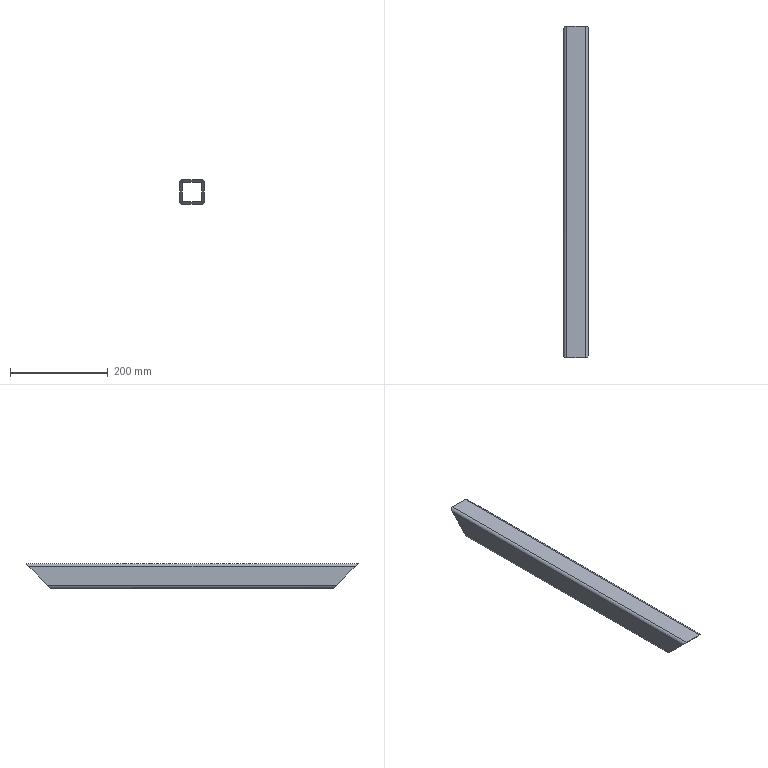Part | SolidWorks | features Extrusion 1, ICE 1 | 1 solid | 18 faces | box 50 x 680 x 50 mm | volume 548072 mm3 | plane 10 | cylinder 8 | commonest cylinder face diameters 2 x4 12 x4
STEP:
#1=CARTESIAN_POINT('',(-20.,674.,6.278));
#2=VERTEX_POINT('',#1);
#3=CARTESIAN_POINT('',(-20.,636.,-31.722));
#4=VERTEX_POINT('',#3);
#5=CARTESIAN_POINT('',(-20.,677.,9.278));
#6=DIRECTION('',(0.,-0.7071,-0.7071));
#7=VECTOR('',#6,1000.);
#8=LINE('',#5,#7);
#9=EDGE_CURVE('',#2,#4,#8,.T.);
#10=ORIENTED_EDGE('',*,*,#9,.F.);
#11=CARTESIAN_POINT('',(-20.,6.,6.278));
#12=VERTEX_POINT('',#11);
#13=CARTESIAN_POINT('',(-20.,680.,6.278));
#14=DIRECTION('',(0.,-1.,0.));
#15=VECTOR('',#14,1000.);
#16=LINE('',#13,#15);
#17=EDGE_CURVE('',#2,#12,#16,.T.);
#18=ORIENTED_EDGE('',*,*,#17,.T.);
#19=CARTESIAN_POINT('',(-20.,44.,-31.722));
#20=VERTEX_POINT('',#19);
#21=CARTESIAN_POINT('',(-20.,343.,-330.722));
#22=DIRECTION('',(0.,-0.7071,0.7071));
#23=VECTOR('',#22,1000.);
#24=LINE('',#21,#23);
#25=EDGE_CURVE('',#20,#12,#24,.T.);
#26=ORIENTED_EDGE('',*,*,#25,.F.);
#27=CARTESIAN_POINT('',(-20.,680.,-31.722));
#28=DIRECTION('',(0.,-1.,0.));
#29=VECTOR('',#28,1000.);
#30=LINE('',#27,#29);
#31=EDGE_CURVE('',#4,#20,#30,.T.);
#32=ORIENTED_EDGE('',*,*,#31,.F.);
#33=EDGE_LOOP('',(#10,#18,#26,#32));
#34=FACE_OUTER_BOUND('',#33,.T.);
#35=CARTESIAN_POINT('',(-20.,680.,6.278));
#36=DIRECTION('',(1.,0.,0.));
#37=DIRECTION('',(0.,0.,-1.));
#38=AXIS2_PLACEMENT_3D('',#35,#36,#37);
#39=PLANE('',#38);
#40=ADVANCED_FACE('',(#34),#39,.T.);
#41=CARTESIAN_POINT('',(-19.,635.,-32.722));
#42=VERTEX_POINT('',#41);
#43=CARTESIAN_POINT('',(-20.,636.,-31.722));
#44=CARTESIAN_POINT('',(-20.,635.414,-32.308));
#45=CARTESIAN_POINT('',(-19.586,635.,-32.722));
#46=CARTESIAN_POINT('',(-19.,635.,-32.722));
#47=(BOUNDED_CURVE()B_SPLINE_CURVE(3,(#43,#44,#45,#46),.UNSPECIFIED.,.F.,.F.)B_SPLINE_CURVE_WITH_KNOTS((4,4),(4.712,6.283),.UNSPECIFIED.)CURVE()GEOMETRIC_REPRESENTATION_ITEM()RATIONAL_B_SPLINE_CURVE((1.,0.8047,0.8047,1.))REPRESENTATION_ITEM(''));
#48=EDGE_CURVE('',#4,#42,#47,.T.);
#49=ORIENTED_EDGE('',*,*,#48,.F.);
#50=ORIENTED_EDGE('',*,*,#31,.T.);
#51=CARTESIAN_POINT('',(-19.,45.,-32.722));
#52=VERTEX_POINT('',#51);
#53=CARTESIAN_POINT('',(-19.,45.,-32.722));
#54=CARTESIAN_POINT('',(-19.586,45.,-32.722));
#55=CARTESIAN_POINT('',(-20.,44.586,-32.308));
#56=CARTESIAN_POINT('',(-20.,44.,-31.722));
#57=(BOUNDED_CURVE()B_SPLINE_CURVE(3,(#53,#54,#55,#56),.UNSPECIFIED.,.F.,.F.)B_SPLINE_CURVE_WITH_KNOTS((4,4),(3.142,4.712),.UNSPECIFIED.)CURVE()GEOMETRIC_REPRESENTATION_ITEM()RATIONAL_B_SPLINE_CURVE((1.,0.8047,0.8047,1.))REPRESENTATION_ITEM(''));
#58=EDGE_CURVE('',#52,#20,#57,.T.);
#59=ORIENTED_EDGE('',*,*,#58,.F.);
#60=CARTESIAN_POINT('',(-19.,680.,-32.722));
#61=DIRECTION('',(0.,-1.,0.));
#62=VECTOR('',#61,1000.);
#63=LINE('',#60,#62);
#64=EDGE_CURVE('',#42,#52,#63,.T.);
#65=ORIENTED_EDGE('',*,*,#64,.F.);
#66=EDGE_LOOP('',(#49,#50,#59,#65));
#67=FACE_OUTER_BOUND('',#66,.T.);
#68=CARTESIAN_POINT('',(-19.,680.,-31.722));
#69=DIRECTION('',(0.,-1.,0.));
#70=DIRECTION('',(0.,0.,-1.));
#71=AXIS2_PLACEMENT_3D('',#68,#69,#70);
#72=CYLINDRICAL_SURFACE('',#71,1.);
#73=ADVANCED_FACE('',(#67),#72,.F.);
#74=CARTESIAN_POINT('',(19.,635.,-32.722));
#75=VERTEX_POINT('',#74);
#76=CARTESIAN_POINT('',(-19.,635.,-32.722));
#77=DIRECTION('',(1.,0.,0.));
#78=VECTOR('',#77,1000.);
#79=LINE('',#76,#78);
#80=EDGE_CURVE('',#42,#75,#79,.T.);
#81=ORIENTED_EDGE('',*,*,#80,.F.);
#82=ORIENTED_EDGE('',*,*,#64,.T.);
#83=CARTESIAN_POINT('',(19.,45.,-32.722));
#84=VERTEX_POINT('',#83);
#85=CARTESIAN_POINT('',(-19.,45.,-32.722));
#86=DIRECTION('',(-1.,0.,0.));
#87=VECTOR('',#86,1000.);
#88=LINE('',#85,#87);
#89=EDGE_CURVE('',#84,#52,#88,.T.);
#90=ORIENTED_EDGE('',*,*,#89,.F.);
#91=CARTESIAN_POINT('',(19.,680.,-32.722));
#92=DIRECTION('',(0.,-1.,0.));
#93=VECTOR('',#92,1000.);
#94=LINE('',#91,#93);
#95=EDGE_CURVE('',#75,#84,#94,.T.);
#96=ORIENTED_EDGE('',*,*,#95,.F.);
#97=EDGE_LOOP('',(#81,#82,#90,#96));
#98=FACE_OUTER_BOUND('',#97,.T.);
#99=CARTESIAN_POINT('',(-19.,680.,-32.722));
#100=DIRECTION('',(0.,0.,1.));
#101=DIRECTION('',(1.,0.,0.));
#102=AXIS2_PLACEMENT_3D('',#99,#100,#101);
#103=PLANE('',#102);
#104=ADVANCED_FACE('',(#98),#103,.T.);
#105=CARTESIAN_POINT('',(20.,636.,-31.722));
#106=VERTEX_POINT('',#105);
#107=CARTESIAN_POINT('',(19.,635.,-32.722));
#108=CARTESIAN_POINT('',(19.586,635.,-32.722));
#109=CARTESIAN_POINT('',(20.,635.414,-32.308));
#110=CARTESIAN_POINT('',(20.,636.,-31.722));
#111=(BOUNDED_CURVE()B_SPLINE_CURVE(3,(#107,#108,#109,#110),.UNSPECIFIED.,.F.,.F.)B_SPLINE_CURVE_WITH_KNOTS((4,4),(0.,1.571),.UNSPECIFIED.)CURVE()GEOMETRIC_REPRESENTATION_ITEM()RATIONAL_B_SPLINE_CURVE((1.,0.8047,0.8047,1.))REPRESENTATION_ITEM(''));
#112=EDGE_CURVE('',#75,#106,#111,.T.);
#113=ORIENTED_EDGE('',*,*,#112,.F.);
#114=ORIENTED_EDGE('',*,*,#95,.T.);
#115=CARTESIAN_POINT('',(20.,44.,-31.722));
#116=VERTEX_POINT('',#115);
#117=CARTESIAN_POINT('',(20.,44.,-31.722));
#118=CARTESIAN_POINT('',(20.,44.586,-32.308));
#119=CARTESIAN_POINT('',(19.586,45.,-32.722));
#120=CARTESIAN_POINT('',(19.,45.,-32.722));
#121=(BOUNDED_CURVE()B_SPLINE_CURVE(3,(#117,#118,#119,#120),.UNSPECIFIED.,.F.,.F.)B_SPLINE_CURVE_WITH_KNOTS((4,4),(1.571,3.142),.UNSPECIFIED.)CURVE()GEOMETRIC_REPRESENTATION_ITEM()RATIONAL_B_SPLINE_CURVE((1.,0.8047,0.8047,1.))REPRESENTATION_ITEM(''));
#122=EDGE_CURVE('',#116,#84,#121,.T.);
#123=ORIENTED_EDGE('',*,*,#122,.F.);
#124=CARTESIAN_POINT('',(20.,680.,-31.722));
#125=DIRECTION('',(0.,-1.,0.));
#126=VECTOR('',#125,1000.);
#127=LINE('',#124,#126);
#128=EDGE_CURVE('',#106,#116,#127,.T.);
#129=ORIENTED_EDGE('',*,*,#128,.F.);
#130=EDGE_LOOP('',(#113,#114,#123,#129));
#131=FACE_OUTER_BOUND('',#130,.T.);
#132=CARTESIAN_POINT('',(19.,680.,-31.722));
#133=DIRECTION('',(0.,-1.,0.));
#134=DIRECTION('',(0.,0.,-1.));
#135=AXIS2_PLACEMENT_3D('',#132,#133,#134);
#136=CYLINDRICAL_SURFACE('',#135,1.);
#137=ADVANCED_FACE('',(#131),#136,.F.);
#138=CARTESIAN_POINT('',(20.,674.,6.278));
#139=VERTEX_POINT('',#138);
#140=CARTESIAN_POINT('',(20.,677.,9.278));
#141=DIRECTION('',(0.,0.7071,0.7071));
#142=VECTOR('',#141,1000.);
#143=LINE('',#140,#142);
#144=EDGE_CURVE('',#106,#139,#143,.T.);
#145=ORIENTED_EDGE('',*,*,#144,.F.);
#146=ORIENTED_EDGE('',*,*,#128,.T.);
#147=CARTESIAN_POINT('',(20.,6.,6.278));
#148=VERTEX_POINT('',#147);
#149=CARTESIAN_POINT('',(20.,343.,-330.722));
#150=DIRECTION('',(0.,0.7071,-0.7071));
#151=VECTOR('',#150,1000.);
#152=LINE('',#149,#151);
#153=EDGE_CURVE('',#148,#116,#152,.T.);
#154=ORIENTED_EDGE('',*,*,#153,.F.);
#155=CARTESIAN_POINT('',(20.,680.,6.278));
#156=DIRECTION('',(0.,-1.,0.));
#157=VECTOR('',#156,1000.);
#158=LINE('',#155,#157);
#159=EDGE_CURVE('',#139,#148,#158,.T.);
#160=ORIENTED_EDGE('',*,*,#159,.F.);
#161=EDGE_LOOP('',(#145,#146,#154,#160));
#162=FACE_OUTER_BOUND('',#161,.T.);
#163=CARTESIAN_POINT('',(20.,680.,6.278));
#164=DIRECTION('',(-1.,0.,0.));
#165=DIRECTION('',(0.,0.,1.));
#166=AXIS2_PLACEMENT_3D('',#163,#164,#165);
#167=PLANE('',#166);
#168=ADVANCED_FACE('',(#162),#167,.T.);
#169=CARTESIAN_POINT('',(19.,675.,7.278));
#170=VERTEX_POINT('',#169);
#171=CARTESIAN_POINT('',(20.,674.,6.278));
#172=CARTESIAN_POINT('',(20.,674.586,6.864));
#173=CARTESIAN_POINT('',(19.586,675.,7.278));
#174=CARTESIAN_POINT('',(19.,675.,7.278));
#175=(BOUNDED_CURVE()B_SPLINE_CURVE(3,(#171,#172,#173,#174),.UNSPECIFIED.,.F.,.F.)B_SPLINE_CURVE_WITH_KNOTS((4,4),(1.571,3.142),.UNSPECIFIED.)CURVE()GEOMETRIC_REPRESENTATION_ITEM()RATIONAL_B_SPLINE_CURVE((1.,0.8047,0.8047,1.))REPRESENTATION_ITEM(''));
#176=EDGE_CURVE('',#139,#170,#175,.T.);
#177=ORIENTED_EDGE('',*,*,#176,.F.);
#178=ORIENTED_EDGE('',*,*,#159,.T.);
#179=CARTESIAN_POINT('',(19.,5.,7.278));
#180=VERTEX_POINT('',#179);
#181=CARTESIAN_POINT('',(19.,5.,7.278));
#182=CARTESIAN_POINT('',(19.586,5.,7.278));
#183=CARTESIAN_POINT('',(20.,5.414,6.864));
#184=CARTESIAN_POINT('',(20.,6.,6.278));
#185=(BOUNDED_CURVE()B_SPLINE_CURVE(3,(#181,#182,#183,#184),.UNSPECIFIED.,.F.,.F.)B_SPLINE_CURVE_WITH_KNOTS((4,4),(0.,1.571),.UNSPECIFIED.)CURVE()GEOMETRIC_REPRESENTATION_ITEM()RATIONAL_B_SPLINE_CURVE((1.,0.8047,0.8047,1.))REPRESENTATION_ITEM(''));
#186=EDGE_CURVE('',#180,#148,#185,.T.);
#187=ORIENTED_EDGE('',*,*,#186,.F.);
#188=CARTESIAN_POINT('',(19.,680.,7.278));
#189=DIRECTION('',(0.,-1.,0.));
#190=VECTOR('',#189,1000.);
#191=LINE('',#188,#190);
#192=EDGE_CURVE('',#170,#180,#191,.T.);
#193=ORIENTED_EDGE('',*,*,#192,.F.);
#194=EDGE_LOOP('',(#177,#178,#187,#193));
#195=FACE_OUTER_BOUND('',#194,.T.);
#196=CARTESIAN_POINT('',(19.,680.,6.278));
#197=DIRECTION('',(0.,-1.,0.));
#198=DIRECTION('',(0.,0.,-1.));
#199=AXIS2_PLACEMENT_3D('',#196,#197,#198);
#200=CYLINDRICAL_SURFACE('',#199,1.);
#201=ADVANCED_FACE('',(#195),#200,.F.);
#202=CARTESIAN_POINT('',(-19.,675.,7.278));
#203=VERTEX_POINT('',#202);
#204=CARTESIAN_POINT('',(-19.,675.,7.278));
#205=DIRECTION('',(-1.,0.,0.));
#206=VECTOR('',#205,1000.);
#207=LINE('',#204,#206);
#208=EDGE_CURVE('',#170,#203,#207,.T.);
#209=ORIENTED_EDGE('',*,*,#208,.F.);
#210=ORIENTED_EDGE('',*,*,#192,.T.);
#211=CARTESIAN_POINT('',(-19.,5.,7.278));
#212=VERTEX_POINT('',#211);
#213=CARTESIAN_POINT('',(-19.,5.,7.278));
#214=DIRECTION('',(1.,0.,0.));
#215=VECTOR('',#214,1000.);
#216=LINE('',#213,#215);
#217=EDGE_CURVE('',#212,#180,#216,.T.);
#218=ORIENTED_EDGE('',*,*,#217,.F.);
#219=CARTESIAN_POINT('',(-19.,680.,7.278));
#220=DIRECTION('',(0.,-1.,0.));
#221=VECTOR('',#220,1000.);
#222=LINE('',#219,#221);
#223=EDGE_CURVE('',#203,#212,#222,.T.);
#224=ORIENTED_EDGE('',*,*,#223,.F.);
#225=EDGE_LOOP('',(#209,#210,#218,#224));
#226=FACE_OUTER_BOUND('',#225,.T.);
#227=CARTESIAN_POINT('',(-19.,680.,7.278));
#228=DIRECTION('',(0.,0.,-1.));
#229=DIRECTION('',(-1.,0.,0.));
#230=AXIS2_PLACEMENT_3D('',#227,#228,#229);
#231=PLANE('',#230);
#232=ADVANCED_FACE('',(#226),#231,.T.);
#233=CARTESIAN_POINT('',(-19.,675.,7.278));
#234=CARTESIAN_POINT('',(-19.586,675.,7.278));
#235=CARTESIAN_POINT('',(-20.,674.586,6.864));
#236=CARTESIAN_POINT('',(-20.,674.,6.278));
#237=(BOUNDED_CURVE()B_SPLINE_CURVE(3,(#233,#234,#235,#236),.UNSPECIFIED.,.F.,.F.)B_SPLINE_CURVE_WITH_KNOTS((4,4),(3.142,4.712),.UNSPECIFIED.)CURVE()GEOMETRIC_REPRESENTATION_ITEM()RATIONAL_B_SPLINE_CURVE((1.,0.8047,0.8047,1.))REPRESENTATION_ITEM(''));
#238=EDGE_CURVE('',#203,#2,#237,.T.);
#239=ORIENTED_EDGE('',*,*,#238,.F.);
#240=ORIENTED_EDGE('',*,*,#223,.T.);
#241=CARTESIAN_POINT('',(-20.,6.,6.278));
#242=CARTESIAN_POINT('',(-20.,5.414,6.864));
#243=CARTESIAN_POINT('',(-19.586,5.,7.278));
#244=CARTESIAN_POINT('',(-19.,5.,7.278));
#245=(BOUNDED_CURVE()B_SPLINE_CURVE(3,(#241,#242,#243,#244),.UNSPECIFIED.,.F.,.F.)B_SPLINE_CURVE_WITH_KNOTS((4,4),(4.712,6.283),.UNSPECIFIED.)CURVE()GEOMETRIC_REPRESENTATION_ITEM()RATIONAL_B_SPLINE_CURVE((1.,0.8047,0.8047,1.))REPRESENTATION_ITEM(''));
#246=EDGE_CURVE('',#12,#212,#245,.T.);
#247=ORIENTED_EDGE('',*,*,#246,.F.);
#248=ORIENTED_EDGE('',*,*,#17,.F.);
#249=EDGE_LOOP('',(#239,#240,#247,#248));
#250=FACE_OUTER_BOUND('',#249,.T.);
#251=CARTESIAN_POINT('',(-19.,680.,6.278));
#252=DIRECTION('',(0.,-1.,0.));
#253=DIRECTION('',(0.,0.,-1.));
#254=AXIS2_PLACEMENT_3D('',#251,#252,#253);
#255=CYLINDRICAL_SURFACE('',#254,1.);
#256=ADVANCED_FACE('',(#250),#255,.F.);
#257=ORIENTED_EDGE('',*,*,#246,.T.);
#258=ORIENTED_EDGE('',*,*,#217,.T.);
#259=ORIENTED_EDGE('',*,*,#186,.T.);
#260=ORIENTED_EDGE('',*,*,#153,.T.);
#261=ORIENTED_EDGE('',*,*,#122,.T.);
#262=ORIENTED_EDGE('',*,*,#89,.T.);
#263=ORIENTED_EDGE('',*,*,#58,.T.);
#264=ORIENTED_EDGE('',*,*,#25,.T.);
#265=EDGE_LOOP('',(#257,#258,#259,#260,#261,#262,#263,#264));
#266=FACE_BOUND('',#265,.T.);
#267=CARTESIAN_POINT('',(-25.,44.,-31.722));
#268=VERTEX_POINT('',#267);
#269=CARTESIAN_POINT('',(-25.,6.,6.278));
#270=VERTEX_POINT('',#269);
#271=CARTESIAN_POINT('',(-25.,0.,12.278));
#272=DIRECTION('',(0.,-0.7071,0.7071));
#273=VECTOR('',#272,1000.);
#274=LINE('',#271,#273);
#275=EDGE_CURVE('',#268,#270,#274,.T.);
#276=ORIENTED_EDGE('',*,*,#275,.F.);
#277=CARTESIAN_POINT('',(-19.,50.,-37.722));
#278=VERTEX_POINT('',#277);
#279=CARTESIAN_POINT('',(-19.,50.,-37.722));
#280=CARTESIAN_POINT('',(-22.515,50.,-37.722));
#281=CARTESIAN_POINT('',(-25.,47.515,-35.237));
#282=CARTESIAN_POINT('',(-25.,44.,-31.722));
#283=(BOUNDED_CURVE()B_SPLINE_CURVE(3,(#279,#280,#281,#282),.UNSPECIFIED.,.F.,.F.)B_SPLINE_CURVE_WITH_KNOTS((4,4),(3.142,4.712),.UNSPECIFIED.)CURVE()GEOMETRIC_REPRESENTATION_ITEM()RATIONAL_B_SPLINE_CURVE((1.,0.8047,0.8047,1.))REPRESENTATION_ITEM(''));
#284=EDGE_CURVE('',#278,#268,#283,.T.);
#285=ORIENTED_EDGE('',*,*,#284,.F.);
#286=CARTESIAN_POINT('',(19.,50.,-37.722));
#287=VERTEX_POINT('',#286);
#288=CARTESIAN_POINT('',(-25.,50.,-37.722));
#289=DIRECTION('',(1.,0.,0.));
#290=VECTOR('',#289,1000.);
#291=LINE('',#288,#290);
#292=EDGE_CURVE('',#278,#287,#291,.T.);
#293=ORIENTED_EDGE('',*,*,#292,.T.);
#294=CARTESIAN_POINT('',(25.,44.,-31.722));
#295=VERTEX_POINT('',#294);
#296=CARTESIAN_POINT('',(25.,44.,-31.722));
#297=CARTESIAN_POINT('',(25.,47.515,-35.237));
#298=CARTESIAN_POINT('',(22.515,50.,-37.722));
#299=CARTESIAN_POINT('',(19.,50.,-37.722));
#300=(BOUNDED_CURVE()B_SPLINE_CURVE(3,(#296,#297,#298,#299),.UNSPECIFIED.,.F.,.F.)B_SPLINE_CURVE_WITH_KNOTS((4,4),(1.571,3.142),.UNSPECIFIED.)CURVE()GEOMETRIC_REPRESENTATION_ITEM()RATIONAL_B_SPLINE_CURVE((1.,0.8047,0.8047,1.))REPRESENTATION_ITEM(''));
#301=EDGE_CURVE('',#295,#287,#300,.T.);
#302=ORIENTED_EDGE('',*,*,#301,.F.);
#303=CARTESIAN_POINT('',(25.,6.,6.278));
#304=VERTEX_POINT('',#303);
#305=CARTESIAN_POINT('',(25.,0.,12.278));
#306=DIRECTION('',(0.,-0.7071,0.7071));
#307=VECTOR('',#306,1000.);
#308=LINE('',#305,#307);
#309=EDGE_CURVE('',#295,#304,#308,.T.);
#310=ORIENTED_EDGE('',*,*,#309,.T.);
#311=CARTESIAN_POINT('',(19.,0.,12.278));
#312=VERTEX_POINT('',#311);
#313=CARTESIAN_POINT('',(19.,0.,12.278));
#314=CARTESIAN_POINT('',(22.515,0.,12.278));
#315=CARTESIAN_POINT('',(25.,2.485,9.793));
#316=CARTESIAN_POINT('',(25.,6.,6.278));
#317=(BOUNDED_CURVE()B_SPLINE_CURVE(3,(#313,#314,#315,#316),.UNSPECIFIED.,.F.,.F.)B_SPLINE_CURVE_WITH_KNOTS((4,4),(0.,1.571),.UNSPECIFIED.)CURVE()GEOMETRIC_REPRESENTATION_ITEM()RATIONAL_B_SPLINE_CURVE((1.,0.8047,0.8047,1.))REPRESENTATION_ITEM(''));
#318=EDGE_CURVE('',#312,#304,#317,.T.);
#319=ORIENTED_EDGE('',*,*,#318,.F.);
#320=CARTESIAN_POINT('',(-19.,0.,12.278));
#321=VERTEX_POINT('',#320);
#322=CARTESIAN_POINT('',(-19.,0.,12.278));
#323=DIRECTION('',(1.,0.,0.));
#324=VECTOR('',#323,1000.);
#325=LINE('',#322,#324);
#326=EDGE_CURVE('',#321,#312,#325,.T.);
#327=ORIENTED_EDGE('',*,*,#326,.F.);
#328=CARTESIAN_POINT('',(-25.,6.,6.278));
#329=CARTESIAN_POINT('',(-25.,2.485,9.793));
#330=CARTESIAN_POINT('',(-22.515,0.,12.278));
#331=CARTESIAN_POINT('',(-19.,0.,12.278));
#332=(BOUNDED_CURVE()B_SPLINE_CURVE(3,(#328,#329,#330,#331),.UNSPECIFIED.,.F.,.F.)B_SPLINE_CURVE_WITH_KNOTS((4,4),(4.712,6.283),.UNSPECIFIED.)CURVE()GEOMETRIC_REPRESENTATION_ITEM()RATIONAL_B_SPLINE_CURVE((1.,0.8047,0.8047,1.))REPRESENTATION_ITEM(''));
#333=EDGE_CURVE('',#270,#321,#332,.T.);
#334=ORIENTED_EDGE('',*,*,#333,.F.);
#335=EDGE_LOOP('',(#276,#285,#293,#302,#310,#319,#327,#334));
#336=FACE_OUTER_BOUND('',#335,.T.);
#337=CARTESIAN_POINT('',(-25.,0.,12.278));
#338=DIRECTION('',(0.,0.7071,0.7071));
#339=DIRECTION('',(0.,-0.7071,0.7071));
#340=AXIS2_PLACEMENT_3D('',#337,#338,#339);
#341=PLANE('',#340);
#342=ADVANCED_FACE('',(#266,#336),#341,.F.);
#343=ORIENTED_EDGE('',*,*,#238,.T.);
#344=ORIENTED_EDGE('',*,*,#9,.T.);
#345=ORIENTED_EDGE('',*,*,#48,.T.);
#346=ORIENTED_EDGE('',*,*,#80,.T.);
#347=ORIENTED_EDGE('',*,*,#112,.T.);
#348=ORIENTED_EDGE('',*,*,#144,.T.);
#349=ORIENTED_EDGE('',*,*,#176,.T.);
#350=ORIENTED_EDGE('',*,*,#208,.T.);
#351=EDGE_LOOP('',(#343,#344,#345,#346,#347,#348,#349,#350));
#352=FACE_BOUND('',#351,.T.);
#353=CARTESIAN_POINT('',(-19.,680.,12.278));
#354=VERTEX_POINT('',#353);
#355=CARTESIAN_POINT('',(19.,680.,12.278));
#356=VERTEX_POINT('',#355);
#357=CARTESIAN_POINT('',(-19.,680.,12.278));
#358=DIRECTION('',(1.,0.,0.));
#359=VECTOR('',#358,1000.);
#360=LINE('',#357,#359);
#361=EDGE_CURVE('',#354,#356,#360,.T.);
#362=ORIENTED_EDGE('',*,*,#361,.T.);
#363=CARTESIAN_POINT('',(25.,674.,6.278));
#364=VERTEX_POINT('',#363);
#365=CARTESIAN_POINT('',(25.,674.,6.278));
#366=CARTESIAN_POINT('',(25.,677.515,9.793));
#367=CARTESIAN_POINT('',(22.515,680.,12.278));
#368=CARTESIAN_POINT('',(19.,680.,12.278));
#369=(BOUNDED_CURVE()B_SPLINE_CURVE(3,(#365,#366,#367,#368),.UNSPECIFIED.,.F.,.F.)B_SPLINE_CURVE_WITH_KNOTS((4,4),(1.571,3.142),.UNSPECIFIED.)CURVE()GEOMETRIC_REPRESENTATION_ITEM()RATIONAL_B_SPLINE_CURVE((1.,0.8047,0.8047,1.))REPRESENTATION_ITEM(''));
#370=EDGE_CURVE('',#364,#356,#369,.T.);
#371=ORIENTED_EDGE('',*,*,#370,.F.);
#372=CARTESIAN_POINT('',(25.,636.,-31.722));
#373=VERTEX_POINT('',#372);
#374=CARTESIAN_POINT('',(25.,630.,-37.722));
#375=DIRECTION('',(0.,-0.7071,-0.7071));
#376=VECTOR('',#375,1000.);
#377=LINE('',#374,#376);
#378=EDGE_CURVE('',#364,#373,#377,.T.);
#379=ORIENTED_EDGE('',*,*,#378,.T.);
#380=CARTESIAN_POINT('',(19.,630.,-37.722));
#381=VERTEX_POINT('',#380);
#382=CARTESIAN_POINT('',(19.,630.,-37.722));
#383=CARTESIAN_POINT('',(22.515,630.,-37.722));
#384=CARTESIAN_POINT('',(25.,632.485,-35.237));
#385=CARTESIAN_POINT('',(25.,636.,-31.722));
#386=(BOUNDED_CURVE()B_SPLINE_CURVE(3,(#382,#383,#384,#385),.UNSPECIFIED.,.F.,.F.)B_SPLINE_CURVE_WITH_KNOTS((4,4),(0.,1.571),.UNSPECIFIED.)CURVE()GEOMETRIC_REPRESENTATION_ITEM()RATIONAL_B_SPLINE_CURVE((1.,0.8047,0.8047,1.))REPRESENTATION_ITEM(''));
#387=EDGE_CURVE('',#381,#373,#386,.T.);
#388=ORIENTED_EDGE('',*,*,#387,.F.);
#389=CARTESIAN_POINT('',(-19.,630.,-37.722));
#390=VERTEX_POINT('',#389);
#391=CARTESIAN_POINT('',(-25.,630.,-37.722));
#392=DIRECTION('',(1.,0.,0.));
#393=VECTOR('',#392,1000.);
#394=LINE('',#391,#393);
#395=EDGE_CURVE('',#390,#381,#394,.T.);
#396=ORIENTED_EDGE('',*,*,#395,.F.);
#397=CARTESIAN_POINT('',(-25.,636.,-31.722));
#398=VERTEX_POINT('',#397);
#399=CARTESIAN_POINT('',(-25.,636.,-31.722));
#400=CARTESIAN_POINT('',(-25.,632.485,-35.237));
#401=CARTESIAN_POINT('',(-22.515,630.,-37.722));
#402=CARTESIAN_POINT('',(-19.,630.,-37.722));
#403=(BOUNDED_CURVE()B_SPLINE_CURVE(3,(#399,#400,#401,#402),.UNSPECIFIED.,.F.,.F.)B_SPLINE_CURVE_WITH_KNOTS((4,4),(4.712,6.283),.UNSPECIFIED.)CURVE()GEOMETRIC_REPRESENTATION_ITEM()RATIONAL_B_SPLINE_CURVE((1.,0.8047,0.8047,1.))REPRESENTATION_ITEM(''));
#404=EDGE_CURVE('',#398,#390,#403,.T.);
#405=ORIENTED_EDGE('',*,*,#404,.F.);
#406=CARTESIAN_POINT('',(-25.,674.,6.278));
#407=VERTEX_POINT('',#406);
#408=CARTESIAN_POINT('',(-25.,630.,-37.722));
#409=DIRECTION('',(0.,-0.7071,-0.7071));
#410=VECTOR('',#409,1000.);
#411=LINE('',#408,#410);
#412=EDGE_CURVE('',#407,#398,#411,.T.);
#413=ORIENTED_EDGE('',*,*,#412,.F.);
#414=CARTESIAN_POINT('',(-19.,680.,12.278));
#415=CARTESIAN_POINT('',(-22.515,680.,12.278));
#416=CARTESIAN_POINT('',(-25.,677.515,9.793));
#417=CARTESIAN_POINT('',(-25.,674.,6.278));
#418=(BOUNDED_CURVE()B_SPLINE_CURVE(3,(#414,#415,#416,#417),.UNSPECIFIED.,.F.,.T.)B_SPLINE_CURVE_WITH_KNOTS((4,4),(3.142,4.712),.UNSPECIFIED.)CURVE()GEOMETRIC_REPRESENTATION_ITEM()RATIONAL_B_SPLINE_CURVE((1.,0.8047,0.8047,1.))REPRESENTATION_ITEM(''));
#419=EDGE_CURVE('',#354,#407,#418,.T.);
#420=ORIENTED_EDGE('',*,*,#419,.F.);
#421=EDGE_LOOP('',(#362,#371,#379,#388,#396,#405,#413,#420));
#422=FACE_OUTER_BOUND('',#421,.T.);
#423=CARTESIAN_POINT('',(-25.,630.,-37.722));
#424=DIRECTION('',(0.,-0.7071,0.7071));
#425=DIRECTION('',(0.,-0.7071,-0.7071));
#426=AXIS2_PLACEMENT_3D('',#423,#424,#425);
#427=PLANE('',#426);
#428=ADVANCED_FACE('',(#352,#422),#427,.F.);
#429=CARTESIAN_POINT('',(-19.,680.,12.278));
#430=DIRECTION('',(0.,-1.,0.));
#431=VECTOR('',#430,1000.);
#432=LINE('',#429,#431);
#433=EDGE_CURVE('',#354,#321,#432,.T.);
#434=ORIENTED_EDGE('',*,*,#433,.F.);
#435=ORIENTED_EDGE('',*,*,#419,.T.);
#436=CARTESIAN_POINT('',(-25.,680.,6.278));
#437=DIRECTION('',(0.,-1.,0.));
#438=VECTOR('',#437,1000.);
#439=LINE('',#436,#438);
#440=EDGE_CURVE('',#407,#270,#439,.T.);
#441=ORIENTED_EDGE('',*,*,#440,.T.);
#442=ORIENTED_EDGE('',*,*,#333,.T.);
#443=EDGE_LOOP('',(#434,#435,#441,#442));
#444=FACE_OUTER_BOUND('',#443,.T.);
#445=CARTESIAN_POINT('',(-19.,680.,6.278));
#446=DIRECTION('',(0.,-1.,0.));
#447=DIRECTION('',(0.,0.,-1.));
#448=AXIS2_PLACEMENT_3D('',#445,#446,#447);
#449=CYLINDRICAL_SURFACE('',#448,6.);
#450=ADVANCED_FACE('',(#444),#449,.T.);
#451=ORIENTED_EDGE('',*,*,#326,.T.);
#452=CARTESIAN_POINT('',(19.,680.,12.278));
#453=DIRECTION('',(0.,-1.,0.));
#454=VECTOR('',#453,1000.);
#455=LINE('',#452,#454);
#456=EDGE_CURVE('',#356,#312,#455,.T.);
#457=ORIENTED_EDGE('',*,*,#456,.F.);
#458=ORIENTED_EDGE('',*,*,#361,.F.);
#459=ORIENTED_EDGE('',*,*,#433,.T.);
#460=EDGE_LOOP('',(#451,#457,#458,#459));
#461=FACE_OUTER_BOUND('',#460,.T.);
#462=CARTESIAN_POINT('',(-19.,680.,12.278));
#463=DIRECTION('',(0.,0.,-1.));
#464=DIRECTION('',(-1.,0.,0.));
#465=AXIS2_PLACEMENT_3D('',#462,#463,#464);
#466=PLANE('',#465);
#467=ADVANCED_FACE('',(#461),#466,.F.);
#468=CARTESIAN_POINT('',(25.,680.,6.278));
#469=DIRECTION('',(0.,-1.,0.));
#470=VECTOR('',#469,1000.);
#471=LINE('',#468,#470);
#472=EDGE_CURVE('',#364,#304,#471,.T.);
#473=ORIENTED_EDGE('',*,*,#472,.F.);
#474=ORIENTED_EDGE('',*,*,#370,.T.);
#475=ORIENTED_EDGE('',*,*,#456,.T.);
#476=ORIENTED_EDGE('',*,*,#318,.T.);
#477=EDGE_LOOP('',(#473,#474,#475,#476));
#478=FACE_OUTER_BOUND('',#477,.T.);
#479=CARTESIAN_POINT('',(19.,680.,6.278));
#480=DIRECTION('',(0.,-1.,0.));
#481=DIRECTION('',(0.,0.,-1.));
#482=AXIS2_PLACEMENT_3D('',#479,#480,#481);
#483=CYLINDRICAL_SURFACE('',#482,6.);
#484=ADVANCED_FACE('',(#478),#483,.T.);
#485=CARTESIAN_POINT('',(25.,680.,-31.722));
#486=DIRECTION('',(0.,-1.,0.));
#487=VECTOR('',#486,1000.);
#488=LINE('',#485,#487);
#489=EDGE_CURVE('',#373,#295,#488,.T.);
#490=ORIENTED_EDGE('',*,*,#489,.F.);
#491=ORIENTED_EDGE('',*,*,#378,.F.);
#492=ORIENTED_EDGE('',*,*,#472,.T.);
#493=ORIENTED_EDGE('',*,*,#309,.F.);
#494=EDGE_LOOP('',(#490,#491,#492,#493));
#495=FACE_OUTER_BOUND('',#494,.T.);
#496=CARTESIAN_POINT('',(25.,680.,6.278));
#497=DIRECTION('',(-1.,0.,0.));
#498=DIRECTION('',(0.,0.,1.));
#499=AXIS2_PLACEMENT_3D('',#496,#497,#498);
#500=PLANE('',#499);
#501=ADVANCED_FACE('',(#495),#500,.F.);
#502=CARTESIAN_POINT('',(19.,680.,-37.722));
#503=DIRECTION('',(0.,-1.,0.));
#504=VECTOR('',#503,1000.);
#505=LINE('',#502,#504);
#506=EDGE_CURVE('',#381,#287,#505,.T.);
#507=ORIENTED_EDGE('',*,*,#506,.F.);
#508=ORIENTED_EDGE('',*,*,#387,.T.);
#509=ORIENTED_EDGE('',*,*,#489,.T.);
#510=ORIENTED_EDGE('',*,*,#301,.T.);
#511=EDGE_LOOP('',(#507,#508,#509,#510));
#512=FACE_OUTER_BOUND('',#511,.T.);
#513=CARTESIAN_POINT('',(19.,680.,-31.722));
#514=DIRECTION('',(0.,-1.,0.));
#515=DIRECTION('',(0.,0.,-1.));
#516=AXIS2_PLACEMENT_3D('',#513,#514,#515);
#517=CYLINDRICAL_SURFACE('',#516,6.);
#518=ADVANCED_FACE('',(#512),#517,.T.);
#519=CARTESIAN_POINT('',(-19.,680.,-37.722));
#520=DIRECTION('',(0.,-1.,0.));
#521=VECTOR('',#520,1000.);
#522=LINE('',#519,#521);
#523=EDGE_CURVE('',#390,#278,#522,.T.);
#524=ORIENTED_EDGE('',*,*,#523,.F.);
#525=ORIENTED_EDGE('',*,*,#395,.T.);
#526=ORIENTED_EDGE('',*,*,#506,.T.);
#527=ORIENTED_EDGE('',*,*,#292,.F.);
#528=EDGE_LOOP('',(#524,#525,#526,#527));
#529=FACE_OUTER_BOUND('',#528,.T.);
#530=CARTESIAN_POINT('',(-19.,680.,-37.722));
#531=DIRECTION('',(0.,0.,1.));
#532=DIRECTION('',(1.,0.,0.));
#533=AXIS2_PLACEMENT_3D('',#530,#531,#532);
#534=PLANE('',#533);
#535=ADVANCED_FACE('',(#529),#534,.F.);
#536=CARTESIAN_POINT('',(-25.,680.,-31.722));
#537=DIRECTION('',(0.,-1.,0.));
#538=VECTOR('',#537,1000.);
#539=LINE('',#536,#538);
#540=EDGE_CURVE('',#398,#268,#539,.T.);
#541=ORIENTED_EDGE('',*,*,#540,.F.);
#542=ORIENTED_EDGE('',*,*,#404,.T.);
#543=ORIENTED_EDGE('',*,*,#523,.T.);
#544=ORIENTED_EDGE('',*,*,#284,.T.);
#545=EDGE_LOOP('',(#541,#542,#543,#544));
#546=FACE_OUTER_BOUND('',#545,.T.);
#547=CARTESIAN_POINT('',(-19.,680.,-31.722));
#548=DIRECTION('',(0.,-1.,0.));
#549=DIRECTION('',(0.,0.,-1.));
#550=AXIS2_PLACEMENT_3D('',#547,#548,#549);
#551=CYLINDRICAL_SURFACE('',#550,6.);
#552=ADVANCED_FACE('',(#546),#551,.T.);
#553=ORIENTED_EDGE('',*,*,#440,.F.);
#554=ORIENTED_EDGE('',*,*,#412,.T.);
#555=ORIENTED_EDGE('',*,*,#540,.T.);
#556=ORIENTED_EDGE('',*,*,#275,.T.);
#557=EDGE_LOOP('',(#553,#554,#555,#556));
#558=FACE_OUTER_BOUND('',#557,.T.);
#559=CARTESIAN_POINT('',(-25.,680.,6.278));
#560=DIRECTION('',(1.,0.,0.));
#561=DIRECTION('',(0.,0.,-1.));
#562=AXIS2_PLACEMENT_3D('',#559,#560,#561);
#563=PLANE('',#562);
#564=ADVANCED_FACE('',(#558),#563,.F.);
#565=CLOSED_SHELL('',(#40,#73,#104,#137,#168,#201,#232,#256,#342,#428,#450,#467,#484,#501,#518,#535,#552,#564));
#566=MANIFOLD_SOLID_BREP('',#565);
#567=CARTESIAN_POINT('',(0.,0.,0.));
#568=DIRECTION('',(0.,0.,1.));
#569=DIRECTION('',(1.,0.,0.));
#570=AXIS2_PLACEMENT_3D('',#567,#568,#569);
#571=(LENGTH_UNIT()NAMED_UNIT(*)SI_UNIT(.MILLI.,.METRE.));
#572=UNCERTAINTY_MEASURE_WITH_UNIT(LENGTH_MEASURE(0.00001),#571,'','');
#573=(NAMED_UNIT(*)PLANE_ANGLE_UNIT()SI_UNIT($,.RADIAN.));
#574=(NAMED_UNIT(*)SI_UNIT($,.STERADIAN.)SOLID_ANGLE_UNIT());
#575=(GEOMETRIC_REPRESENTATION_CONTEXT(3)GLOBAL_UNCERTAINTY_ASSIGNED_CONTEXT((#572))GLOBAL_UNIT_ASSIGNED_CONTEXT((#571,#573,#574))REPRESENTATION_CONTEXT('',''));
#576=ADVANCED_BREP_SHAPE_REPRESENTATION('',(#566,#570),#575);